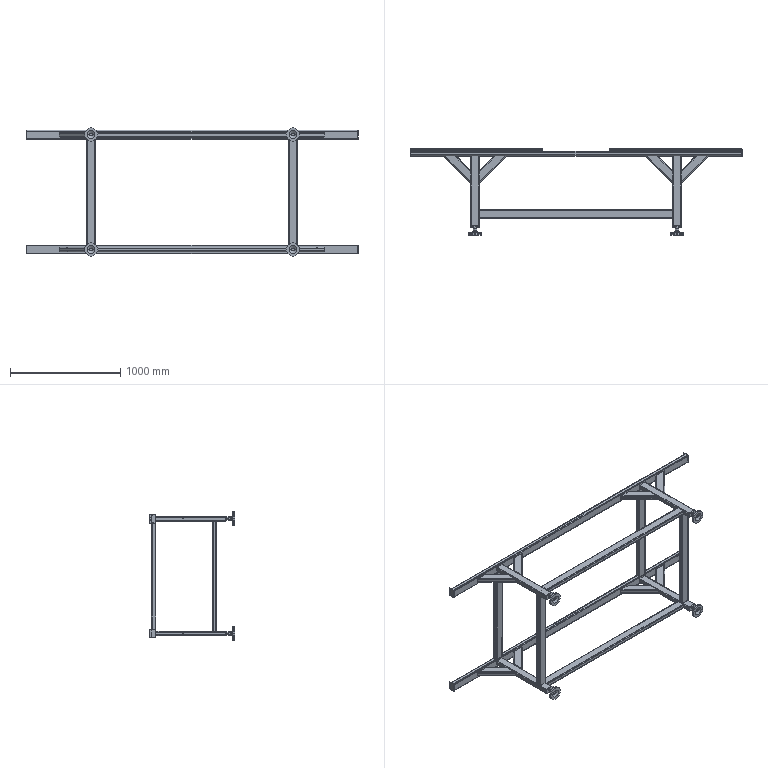Part | SolidWorks | features ReferencePattern 6, LocalLPattern 2 | 34 solids | 778 faces | box 3010 x 778.6 x 1163 mm | volume 17961198 mm3 | plane 382 | cylinder 292 | cone 104 | commonest cylinder face diameters 8 x80 16 x80 7 x36 11 x36 2.933 x20 20 x16